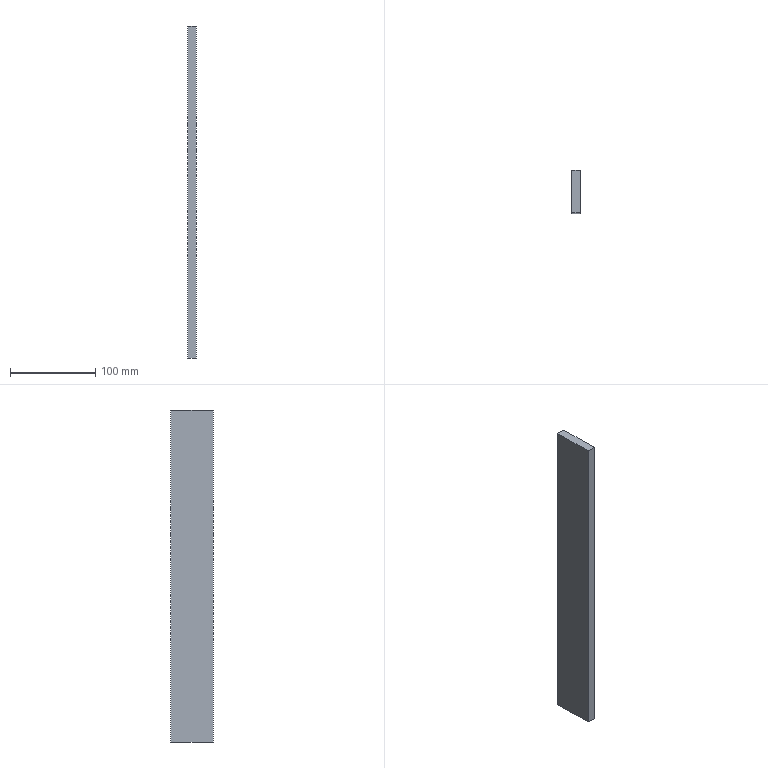Part | NX | features solid 2 | 1 solid | 6 faces | box 10 x 50 x 390 mm | volume 195000 mm3 | plane 6
STEP:
#1=CARTESIAN_POINT('',(-1595.,-830.,200.));
#2=VERTEX_POINT('',#1);
#3=CARTESIAN_POINT('',(-1595.,-780.,200.));
#4=VERTEX_POINT('',#3);
#5=CARTESIAN_POINT('',(-1595.,-830.,200.));
#6=DIRECTION('',(0.,-1.,0.));
#7=VECTOR('',#6,1000.);
#8=LINE('',#5,#7);
#9=EDGE_CURVE('',#2,#4,#8,.F.);
#10=ORIENTED_EDGE('',*,*,#9,.F.);
#11=CARTESIAN_POINT('',(-1595.,-830.,-190.));
#12=VERTEX_POINT('',#11);
#13=CARTESIAN_POINT('',(-1595.,-830.,160.));
#14=DIRECTION('',(0.,0.,-1.));
#15=VECTOR('',#14,1000.);
#16=LINE('',#13,#15);
#17=EDGE_CURVE('',#2,#12,#16,.T.);
#18=ORIENTED_EDGE('',*,*,#17,.T.);
#19=CARTESIAN_POINT('',(-1595.,-780.,-190.));
#20=VERTEX_POINT('',#19);
#21=CARTESIAN_POINT('',(-1595.,-830.,-190.));
#22=DIRECTION('',(0.,1.,0.));
#23=VECTOR('',#22,1000.);
#24=LINE('',#21,#23);
#25=EDGE_CURVE('',#12,#20,#24,.T.);
#26=ORIENTED_EDGE('',*,*,#25,.T.);
#27=CARTESIAN_POINT('',(-1595.,-780.,160.));
#28=DIRECTION('',(0.,0.,1.));
#29=VECTOR('',#28,1000.);
#30=LINE('',#27,#29);
#31=EDGE_CURVE('',#4,#20,#30,.F.);
#32=ORIENTED_EDGE('',*,*,#31,.F.);
#33=EDGE_LOOP('',(#10,#18,#26,#32));
#34=FACE_BOUND('',#33,.T.);
#35=CARTESIAN_POINT('',(-1595.,-830.,160.));
#36=DIRECTION('',(1.,0.,0.));
#37=DIRECTION('',(0.,0.,-1.));
#38=AXIS2_PLACEMENT_3D('',#35,#36,#37);
#39=PLANE('',#38);
#40=ADVANCED_FACE('',(#34),#39,.T.);
#41=ORIENTED_EDGE('',*,*,#25,.F.);
#42=CARTESIAN_POINT('',(-1605.,-830.,-190.));
#43=VERTEX_POINT('',#42);
#44=CARTESIAN_POINT('',(-1595.,-830.,-190.));
#45=DIRECTION('',(1.,0.,0.));
#46=VECTOR('',#45,1000.);
#47=LINE('',#44,#46);
#48=EDGE_CURVE('',#12,#43,#47,.F.);
#49=ORIENTED_EDGE('',*,*,#48,.T.);
#50=CARTESIAN_POINT('',(-1605.,-780.,-190.));
#51=VERTEX_POINT('',#50);
#52=CARTESIAN_POINT('',(-1605.,-830.,-190.));
#53=DIRECTION('',(0.,-1.,0.));
#54=VECTOR('',#53,1000.);
#55=LINE('',#52,#54);
#56=EDGE_CURVE('',#43,#51,#55,.F.);
#57=ORIENTED_EDGE('',*,*,#56,.T.);
#58=CARTESIAN_POINT('',(-1595.,-780.,-190.));
#59=DIRECTION('',(1.,0.,0.));
#60=VECTOR('',#59,1000.);
#61=LINE('',#58,#60);
#62=EDGE_CURVE('',#20,#51,#61,.F.);
#63=ORIENTED_EDGE('',*,*,#62,.F.);
#64=EDGE_LOOP('',(#41,#49,#57,#63));
#65=FACE_BOUND('',#64,.T.);
#66=CARTESIAN_POINT('',(-1595.,-830.,-190.));
#67=DIRECTION('',(0.,0.,-1.));
#68=DIRECTION('',(-1.,0.,0.));
#69=AXIS2_PLACEMENT_3D('',#66,#67,#68);
#70=PLANE('',#69);
#71=ADVANCED_FACE('',(#65),#70,.T.);
#72=ORIENTED_EDGE('',*,*,#56,.F.);
#73=CARTESIAN_POINT('',(-1605.,-830.,200.));
#74=VERTEX_POINT('',#73);
#75=CARTESIAN_POINT('',(-1605.,-830.,160.));
#76=DIRECTION('',(0.,0.,-1.));
#77=VECTOR('',#76,1000.);
#78=LINE('',#75,#77);
#79=EDGE_CURVE('',#74,#43,#78,.T.);
#80=ORIENTED_EDGE('',*,*,#79,.F.);
#81=CARTESIAN_POINT('',(-1605.,-780.,200.));
#82=VERTEX_POINT('',#81);
#83=CARTESIAN_POINT('',(-1605.,-830.,200.));
#84=DIRECTION('',(0.,1.,0.));
#85=VECTOR('',#84,1000.);
#86=LINE('',#83,#85);
#87=EDGE_CURVE('',#74,#82,#86,.T.);
#88=ORIENTED_EDGE('',*,*,#87,.T.);
#89=CARTESIAN_POINT('',(-1605.,-780.,160.));
#90=DIRECTION('',(0.,0.,1.));
#91=VECTOR('',#90,1000.);
#92=LINE('',#89,#91);
#93=EDGE_CURVE('',#82,#51,#92,.F.);
#94=ORIENTED_EDGE('',*,*,#93,.T.);
#95=EDGE_LOOP('',(#72,#80,#88,#94));
#96=FACE_BOUND('',#95,.T.);
#97=CARTESIAN_POINT('',(-1605.,-830.,160.));
#98=DIRECTION('',(1.,0.,0.));
#99=DIRECTION('',(0.,0.,-1.));
#100=AXIS2_PLACEMENT_3D('',#97,#98,#99);
#101=PLANE('',#100);
#102=ADVANCED_FACE('',(#96),#101,.F.);
#103=CARTESIAN_POINT('',(-1595.,-830.,200.));
#104=DIRECTION('',(-1.,0.,0.));
#105=VECTOR('',#104,1000.);
#106=LINE('',#103,#105);
#107=EDGE_CURVE('',#2,#74,#106,.T.);
#108=ORIENTED_EDGE('',*,*,#107,.F.);
#109=ORIENTED_EDGE('',*,*,#9,.T.);
#110=CARTESIAN_POINT('',(-1595.,-780.,200.));
#111=DIRECTION('',(-1.,0.,0.));
#112=VECTOR('',#111,1000.);
#113=LINE('',#110,#112);
#114=EDGE_CURVE('',#4,#82,#113,.T.);
#115=ORIENTED_EDGE('',*,*,#114,.T.);
#116=ORIENTED_EDGE('',*,*,#87,.F.);
#117=EDGE_LOOP('',(#108,#109,#115,#116));
#118=FACE_BOUND('',#117,.T.);
#119=CARTESIAN_POINT('',(-1595.,-830.,200.));
#120=DIRECTION('',(0.,0.,-1.));
#121=DIRECTION('',(-1.,0.,0.));
#122=AXIS2_PLACEMENT_3D('',#119,#120,#121);
#123=PLANE('',#122);
#124=ADVANCED_FACE('',(#118),#123,.F.);
#125=ORIENTED_EDGE('',*,*,#93,.F.);
#126=ORIENTED_EDGE('',*,*,#114,.F.);
#127=ORIENTED_EDGE('',*,*,#31,.T.);
#128=ORIENTED_EDGE('',*,*,#62,.T.);
#129=EDGE_LOOP('',(#125,#126,#127,#128));
#130=FACE_BOUND('',#129,.T.);
#131=CARTESIAN_POINT('',(-1595.,-780.,160.));
#132=DIRECTION('',(0.,-1.,0.));
#133=DIRECTION('',(0.,0.,1.));
#134=AXIS2_PLACEMENT_3D('',#131,#132,#133);
#135=PLANE('',#134);
#136=ADVANCED_FACE('',(#130),#135,.F.);
#137=ORIENTED_EDGE('',*,*,#79,.T.);
#138=ORIENTED_EDGE('',*,*,#48,.F.);
#139=ORIENTED_EDGE('',*,*,#17,.F.);
#140=ORIENTED_EDGE('',*,*,#107,.T.);
#141=EDGE_LOOP('',(#137,#138,#139,#140));
#142=FACE_BOUND('',#141,.T.);
#143=CARTESIAN_POINT('',(-1595.,-830.,160.));
#144=DIRECTION('',(0.,-1.,0.));
#145=DIRECTION('',(0.,0.,1.));
#146=AXIS2_PLACEMENT_3D('',#143,#144,#145);
#147=PLANE('',#146);
#148=ADVANCED_FACE('',(#142),#147,.T.);
#149=CLOSED_SHELL('',(#40,#71,#102,#124,#136,#148));
#150=MANIFOLD_SOLID_BREP('',#149);
#151=(LENGTH_UNIT()NAMED_UNIT(*)SI_UNIT(.MILLI.,.METRE.));
#152=UNCERTAINTY_MEASURE_WITH_UNIT(LENGTH_MEASURE(0.00001),#151,'','');
#153=(NAMED_UNIT(*)PLANE_ANGLE_UNIT()SI_UNIT($,.RADIAN.));
#154=(NAMED_UNIT(*)SI_UNIT($,.STERADIAN.)SOLID_ANGLE_UNIT());
#155=(GEOMETRIC_REPRESENTATION_CONTEXT(3)GLOBAL_UNCERTAINTY_ASSIGNED_CONTEXT((#152))GLOBAL_UNIT_ASSIGNED_CONTEXT((#151,#153,#154))REPRESENTATION_CONTEXT('',''));
#156=ADVANCED_BREP_SHAPE_REPRESENTATION('',(#150),#155);